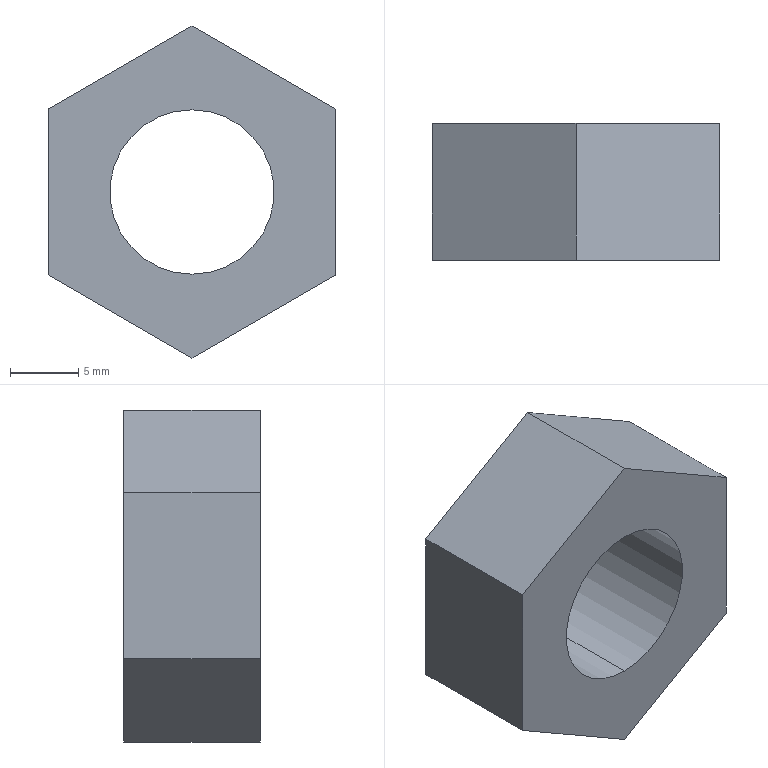Part | SolidWorks | features Extrusion 1, HoleWzd 1 | 1 solid | 10 faces | box 21 x 10 x 24.249 mm | volume 2688 mm3 | plane 8 | cylinder 2 | commonest cylinder face diameters 12 x2
STEP:
#1=CARTESIAN_POINT('',(0.,0.,-6.));
#2=VERTEX_POINT('',#1);
#3=CARTESIAN_POINT('',(0.,0.,6.));
#4=VERTEX_POINT('',#3);
#5=CARTESIAN_POINT('',(0.,0.,0.));
#6=DIRECTION('',(0.,1.,0.));
#7=DIRECTION('',(0.,0.,1.));
#8=AXIS2_PLACEMENT_3D('',#5,#6,#7);
#9=CIRCLE('',#8,6.);
#10=EDGE_CURVE('',#2,#4,#9,.T.);
#11=ORIENTED_EDGE('',*,*,#10,.F.);
#12=CARTESIAN_POINT('',(0.,10.,-6.));
#13=VERTEX_POINT('',#12);
#14=CARTESIAN_POINT('',(0.,10.,-6.));
#15=DIRECTION('',(0.,1.,0.));
#16=VECTOR('',#15,1000.);
#17=LINE('',#14,#16);
#18=EDGE_CURVE('',#2,#13,#17,.T.);
#19=ORIENTED_EDGE('',*,*,#18,.T.);
#20=CARTESIAN_POINT('',(0.,10.,6.));
#21=VERTEX_POINT('',#20);
#22=CARTESIAN_POINT('',(0.,10.,0.));
#23=DIRECTION('',(0.,1.,0.));
#24=DIRECTION('',(0.,0.,1.));
#25=AXIS2_PLACEMENT_3D('',#22,#23,#24);
#26=CIRCLE('',#25,6.);
#27=EDGE_CURVE('',#13,#21,#26,.T.);
#28=ORIENTED_EDGE('',*,*,#27,.T.);
#29=CARTESIAN_POINT('',(0.,10.,6.));
#30=DIRECTION('',(0.,1.,0.));
#31=VECTOR('',#30,1000.);
#32=LINE('',#29,#31);
#33=EDGE_CURVE('',#4,#21,#32,.T.);
#34=ORIENTED_EDGE('',*,*,#33,.F.);
#35=EDGE_LOOP('',(#11,#19,#28,#34));
#36=FACE_OUTER_BOUND('',#35,.T.);
#37=CARTESIAN_POINT('',(0.,10.,0.));
#38=DIRECTION('',(0.,1.,0.));
#39=DIRECTION('',(0.,0.,1.));
#40=AXIS2_PLACEMENT_3D('',#37,#38,#39);
#41=CYLINDRICAL_SURFACE('',#40,6.);
#42=ADVANCED_FACE('',(#36),#41,.F.);
#43=CARTESIAN_POINT('',(10.5,0.,-6.062));
#44=VERTEX_POINT('',#43);
#45=CARTESIAN_POINT('',(0.,0.,-12.124));
#46=VERTEX_POINT('',#45);
#47=CARTESIAN_POINT('',(10.5,0.,-6.062));
#48=DIRECTION('',(-0.866,0.,-0.5));
#49=VECTOR('',#48,1000.);
#50=LINE('',#47,#49);
#51=EDGE_CURVE('',#44,#46,#50,.T.);
#52=ORIENTED_EDGE('',*,*,#51,.T.);
#53=CARTESIAN_POINT('',(0.,10.,-12.124));
#54=VERTEX_POINT('',#53);
#55=CARTESIAN_POINT('',(0.,10.,-12.124));
#56=DIRECTION('',(0.,-1.,0.));
#57=VECTOR('',#56,1000.);
#58=LINE('',#55,#57);
#59=EDGE_CURVE('',#54,#46,#58,.T.);
#60=ORIENTED_EDGE('',*,*,#59,.F.);
#61=CARTESIAN_POINT('',(10.5,10.,-6.062));
#62=VERTEX_POINT('',#61);
#63=CARTESIAN_POINT('',(10.5,10.,-6.062));
#64=DIRECTION('',(-0.866,0.,-0.5));
#65=VECTOR('',#64,1000.);
#66=LINE('',#63,#65);
#67=EDGE_CURVE('',#62,#54,#66,.T.);
#68=ORIENTED_EDGE('',*,*,#67,.F.);
#69=CARTESIAN_POINT('',(10.5,10.,-6.062));
#70=DIRECTION('',(0.,-1.,0.));
#71=VECTOR('',#70,1000.);
#72=LINE('',#69,#71);
#73=EDGE_CURVE('',#62,#44,#72,.T.);
#74=ORIENTED_EDGE('',*,*,#73,.T.);
#75=EDGE_LOOP('',(#52,#60,#68,#74));
#76=FACE_OUTER_BOUND('',#75,.T.);
#77=CARTESIAN_POINT('',(10.5,10.,-6.062));
#78=DIRECTION('',(-0.5,0.,0.866));
#79=DIRECTION('',(0.866,0.,0.5));
#80=AXIS2_PLACEMENT_3D('',#77,#78,#79);
#81=PLANE('',#80);
#82=ADVANCED_FACE('',(#76),#81,.F.);
#83=CARTESIAN_POINT('',(-10.5,0.,-6.062));
#84=VERTEX_POINT('',#83);
#85=CARTESIAN_POINT('',(0.,0.,-12.124));
#86=DIRECTION('',(-0.866,0.,0.5));
#87=VECTOR('',#86,1000.);
#88=LINE('',#85,#87);
#89=EDGE_CURVE('',#46,#84,#88,.T.);
#90=ORIENTED_EDGE('',*,*,#89,.T.);
#91=CARTESIAN_POINT('',(-10.5,10.,-6.062));
#92=VERTEX_POINT('',#91);
#93=CARTESIAN_POINT('',(-10.5,10.,-6.062));
#94=DIRECTION('',(0.,-1.,0.));
#95=VECTOR('',#94,1000.);
#96=LINE('',#93,#95);
#97=EDGE_CURVE('',#92,#84,#96,.T.);
#98=ORIENTED_EDGE('',*,*,#97,.F.);
#99=CARTESIAN_POINT('',(0.,10.,-12.124));
#100=DIRECTION('',(-0.866,0.,0.5));
#101=VECTOR('',#100,1000.);
#102=LINE('',#99,#101);
#103=EDGE_CURVE('',#54,#92,#102,.T.);
#104=ORIENTED_EDGE('',*,*,#103,.F.);
#105=ORIENTED_EDGE('',*,*,#59,.T.);
#106=EDGE_LOOP('',(#90,#98,#104,#105));
#107=FACE_OUTER_BOUND('',#106,.T.);
#108=CARTESIAN_POINT('',(0.,10.,-12.124));
#109=DIRECTION('',(0.5,0.,0.866));
#110=DIRECTION('',(0.866,0.,-0.5));
#111=AXIS2_PLACEMENT_3D('',#108,#109,#110);
#112=PLANE('',#111);
#113=ADVANCED_FACE('',(#107),#112,.F.);
#114=CARTESIAN_POINT('',(-10.5,0.,6.062));
#115=VERTEX_POINT('',#114);
#116=CARTESIAN_POINT('',(-10.5,0.,-6.062));
#117=DIRECTION('',(0.,0.,1.));
#118=VECTOR('',#117,1000.);
#119=LINE('',#116,#118);
#120=EDGE_CURVE('',#84,#115,#119,.T.);
#121=ORIENTED_EDGE('',*,*,#120,.T.);
#122=CARTESIAN_POINT('',(-10.5,10.,6.062));
#123=VERTEX_POINT('',#122);
#124=CARTESIAN_POINT('',(-10.5,10.,6.062));
#125=DIRECTION('',(0.,-1.,0.));
#126=VECTOR('',#125,1000.);
#127=LINE('',#124,#126);
#128=EDGE_CURVE('',#123,#115,#127,.T.);
#129=ORIENTED_EDGE('',*,*,#128,.F.);
#130=CARTESIAN_POINT('',(-10.5,10.,-6.062));
#131=DIRECTION('',(0.,0.,1.));
#132=VECTOR('',#131,1000.);
#133=LINE('',#130,#132);
#134=EDGE_CURVE('',#92,#123,#133,.T.);
#135=ORIENTED_EDGE('',*,*,#134,.F.);
#136=ORIENTED_EDGE('',*,*,#97,.T.);
#137=EDGE_LOOP('',(#121,#129,#135,#136));
#138=FACE_OUTER_BOUND('',#137,.T.);
#139=CARTESIAN_POINT('',(-10.5,10.,-6.062));
#140=DIRECTION('',(1.,0.,0.));
#141=DIRECTION('',(0.,0.,-1.));
#142=AXIS2_PLACEMENT_3D('',#139,#140,#141);
#143=PLANE('',#142);
#144=ADVANCED_FACE('',(#138),#143,.F.);
#145=CARTESIAN_POINT('',(0.,0.,12.124));
#146=VERTEX_POINT('',#145);
#147=CARTESIAN_POINT('',(-10.5,0.,6.062));
#148=DIRECTION('',(0.866,0.,0.5));
#149=VECTOR('',#148,1000.);
#150=LINE('',#147,#149);
#151=EDGE_CURVE('',#115,#146,#150,.T.);
#152=ORIENTED_EDGE('',*,*,#151,.T.);
#153=CARTESIAN_POINT('',(0.,10.,12.124));
#154=VERTEX_POINT('',#153);
#155=CARTESIAN_POINT('',(0.,10.,12.124));
#156=DIRECTION('',(0.,-1.,0.));
#157=VECTOR('',#156,1000.);
#158=LINE('',#155,#157);
#159=EDGE_CURVE('',#154,#146,#158,.T.);
#160=ORIENTED_EDGE('',*,*,#159,.F.);
#161=CARTESIAN_POINT('',(-10.5,10.,6.062));
#162=DIRECTION('',(0.866,0.,0.5));
#163=VECTOR('',#162,1000.);
#164=LINE('',#161,#163);
#165=EDGE_CURVE('',#123,#154,#164,.T.);
#166=ORIENTED_EDGE('',*,*,#165,.F.);
#167=ORIENTED_EDGE('',*,*,#128,.T.);
#168=EDGE_LOOP('',(#152,#160,#166,#167));
#169=FACE_OUTER_BOUND('',#168,.T.);
#170=CARTESIAN_POINT('',(-10.5,10.,6.062));
#171=DIRECTION('',(0.5,0.,-0.866));
#172=DIRECTION('',(-0.866,0.,-0.5));
#173=AXIS2_PLACEMENT_3D('',#170,#171,#172);
#174=PLANE('',#173);
#175=ADVANCED_FACE('',(#169),#174,.F.);
#176=CARTESIAN_POINT('',(10.5,0.,6.062));
#177=VERTEX_POINT('',#176);
#178=CARTESIAN_POINT('',(0.,0.,12.124));
#179=DIRECTION('',(0.866,0.,-0.5));
#180=VECTOR('',#179,1000.);
#181=LINE('',#178,#180);
#182=EDGE_CURVE('',#146,#177,#181,.T.);
#183=ORIENTED_EDGE('',*,*,#182,.T.);
#184=CARTESIAN_POINT('',(10.5,10.,6.062));
#185=VERTEX_POINT('',#184);
#186=CARTESIAN_POINT('',(10.5,10.,6.062));
#187=DIRECTION('',(0.,-1.,0.));
#188=VECTOR('',#187,1000.);
#189=LINE('',#186,#188);
#190=EDGE_CURVE('',#185,#177,#189,.T.);
#191=ORIENTED_EDGE('',*,*,#190,.F.);
#192=CARTESIAN_POINT('',(0.,10.,12.124));
#193=DIRECTION('',(0.866,0.,-0.5));
#194=VECTOR('',#193,1000.);
#195=LINE('',#192,#194);
#196=EDGE_CURVE('',#154,#185,#195,.T.);
#197=ORIENTED_EDGE('',*,*,#196,.F.);
#198=ORIENTED_EDGE('',*,*,#159,.T.);
#199=EDGE_LOOP('',(#183,#191,#197,#198));
#200=FACE_OUTER_BOUND('',#199,.T.);
#201=CARTESIAN_POINT('',(0.,10.,12.124));
#202=DIRECTION('',(-0.5,0.,-0.866));
#203=DIRECTION('',(-0.866,0.,0.5));
#204=AXIS2_PLACEMENT_3D('',#201,#202,#203);
#205=PLANE('',#204);
#206=ADVANCED_FACE('',(#200),#205,.F.);
#207=CARTESIAN_POINT('',(10.5,0.,6.062));
#208=DIRECTION('',(0.,0.,-1.));
#209=VECTOR('',#208,1000.);
#210=LINE('',#207,#209);
#211=EDGE_CURVE('',#177,#44,#210,.T.);
#212=ORIENTED_EDGE('',*,*,#211,.T.);
#213=ORIENTED_EDGE('',*,*,#73,.F.);
#214=CARTESIAN_POINT('',(10.5,10.,6.062));
#215=DIRECTION('',(0.,0.,-1.));
#216=VECTOR('',#215,1000.);
#217=LINE('',#214,#216);
#218=EDGE_CURVE('',#185,#62,#217,.T.);
#219=ORIENTED_EDGE('',*,*,#218,.F.);
#220=ORIENTED_EDGE('',*,*,#190,.T.);
#221=EDGE_LOOP('',(#212,#213,#219,#220));
#222=FACE_OUTER_BOUND('',#221,.T.);
#223=CARTESIAN_POINT('',(10.5,10.,6.062));
#224=DIRECTION('',(-1.,0.,0.));
#225=DIRECTION('',(0.,0.,1.));
#226=AXIS2_PLACEMENT_3D('',#223,#224,#225);
#227=PLANE('',#226);
#228=ADVANCED_FACE('',(#222),#227,.F.);
#229=CARTESIAN_POINT('',(0.,10.,0.));
#230=DIRECTION('',(0.,1.,0.));
#231=DIRECTION('',(0.,0.,1.));
#232=AXIS2_PLACEMENT_3D('',#229,#230,#231);
#233=CIRCLE('',#232,6.);
#234=EDGE_CURVE('',#21,#13,#233,.T.);
#235=ORIENTED_EDGE('',*,*,#234,.F.);
#236=ORIENTED_EDGE('',*,*,#27,.F.);
#237=EDGE_LOOP('',(#235,#236));
#238=FACE_BOUND('',#237,.T.);
#239=ORIENTED_EDGE('',*,*,#67,.T.);
#240=ORIENTED_EDGE('',*,*,#103,.T.);
#241=ORIENTED_EDGE('',*,*,#134,.T.);
#242=ORIENTED_EDGE('',*,*,#165,.T.);
#243=ORIENTED_EDGE('',*,*,#196,.T.);
#244=ORIENTED_EDGE('',*,*,#218,.T.);
#245=EDGE_LOOP('',(#239,#240,#241,#242,#243,#244));
#246=FACE_OUTER_BOUND('',#245,.T.);
#247=CARTESIAN_POINT('',(0.,10.,0.));
#248=DIRECTION('',(0.,1.,0.));
#249=DIRECTION('',(0.,0.,1.));
#250=AXIS2_PLACEMENT_3D('',#247,#248,#249);
#251=PLANE('',#250);
#252=ADVANCED_FACE('',(#238,#246),#251,.T.);
#253=CARTESIAN_POINT('',(0.,0.,0.));
#254=DIRECTION('',(0.,1.,0.));
#255=DIRECTION('',(0.,0.,1.));
#256=AXIS2_PLACEMENT_3D('',#253,#254,#255);
#257=CIRCLE('',#256,6.);
#258=EDGE_CURVE('',#4,#2,#257,.T.);
#259=ORIENTED_EDGE('',*,*,#258,.T.);
#260=ORIENTED_EDGE('',*,*,#10,.T.);
#261=EDGE_LOOP('',(#259,#260));
#262=FACE_BOUND('',#261,.T.);
#263=ORIENTED_EDGE('',*,*,#51,.F.);
#264=ORIENTED_EDGE('',*,*,#211,.F.);
#265=ORIENTED_EDGE('',*,*,#182,.F.);
#266=ORIENTED_EDGE('',*,*,#151,.F.);
#267=ORIENTED_EDGE('',*,*,#120,.F.);
#268=ORIENTED_EDGE('',*,*,#89,.F.);
#269=EDGE_LOOP('',(#263,#264,#265,#266,#267,#268));
#270=FACE_OUTER_BOUND('',#269,.T.);
#271=CARTESIAN_POINT('',(0.,0.,0.));
#272=DIRECTION('',(0.,1.,0.));
#273=DIRECTION('',(0.,0.,1.));
#274=AXIS2_PLACEMENT_3D('',#271,#272,#273);
#275=PLANE('',#274);
#276=ADVANCED_FACE('',(#262,#270),#275,.F.);
#277=ORIENTED_EDGE('',*,*,#18,.F.);
#278=ORIENTED_EDGE('',*,*,#258,.F.);
#279=ORIENTED_EDGE('',*,*,#33,.T.);
#280=ORIENTED_EDGE('',*,*,#234,.T.);
#281=EDGE_LOOP('',(#277,#278,#279,#280));
#282=FACE_OUTER_BOUND('',#281,.T.);
#283=CARTESIAN_POINT('',(0.,10.,0.));
#284=DIRECTION('',(0.,1.,0.));
#285=DIRECTION('',(0.,0.,1.));
#286=AXIS2_PLACEMENT_3D('',#283,#284,#285);
#287=CYLINDRICAL_SURFACE('',#286,6.);
#288=ADVANCED_FACE('',(#282),#287,.F.);
#289=CLOSED_SHELL('',(#42,#82,#113,#144,#175,#206,#228,#252,#276,#288));
#290=MANIFOLD_SOLID_BREP('',#289);
#291=CARTESIAN_POINT('',(0.,0.,0.));
#292=DIRECTION('',(0.,0.,1.));
#293=DIRECTION('',(1.,0.,0.));
#294=AXIS2_PLACEMENT_3D('',#291,#292,#293);
#295=(LENGTH_UNIT()NAMED_UNIT(*)SI_UNIT(.MILLI.,.METRE.));
#296=UNCERTAINTY_MEASURE_WITH_UNIT(LENGTH_MEASURE(0.00001),#295,'','');
#297=(NAMED_UNIT(*)PLANE_ANGLE_UNIT()SI_UNIT($,.RADIAN.));
#298=(NAMED_UNIT(*)SI_UNIT($,.STERADIAN.)SOLID_ANGLE_UNIT());
#299=(GEOMETRIC_REPRESENTATION_CONTEXT(3)GLOBAL_UNCERTAINTY_ASSIGNED_CONTEXT((#296))GLOBAL_UNIT_ASSIGNED_CONTEXT((#295,#297,#298))REPRESENTATION_CONTEXT('',''));
#300=ADVANCED_BREP_SHAPE_REPRESENTATION('',(#290,#294),#299);